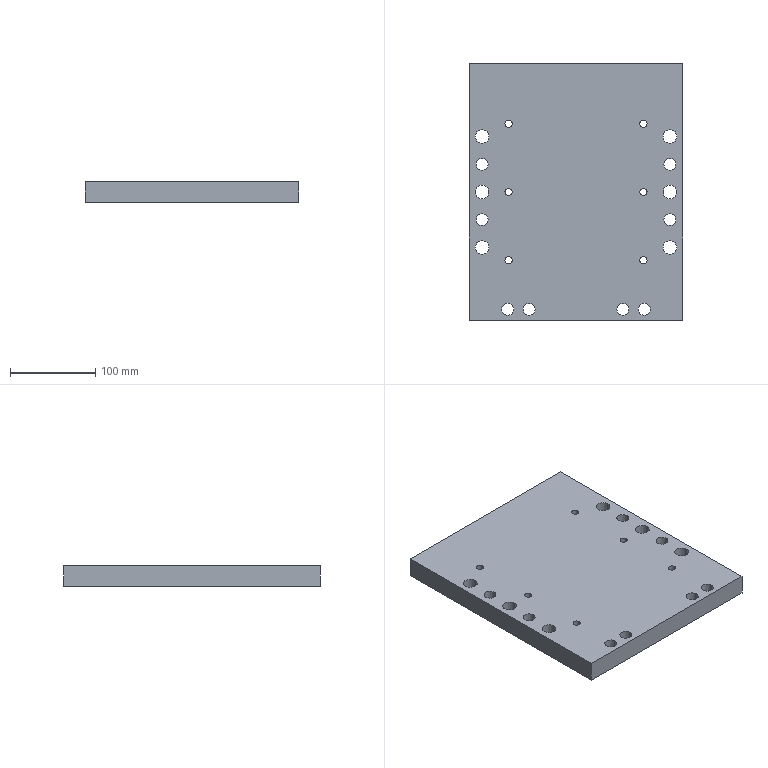Part | STEP file | MAT TRUOT DAU BUA CO LOGO | 1 solid | 46 faces | box 250 x 300 x 24 mm | volume 1733556 mm3 | cylinder 40 | plane 6 | commonest cylinder face diameters 14 x16 8.376 x12 16 x12